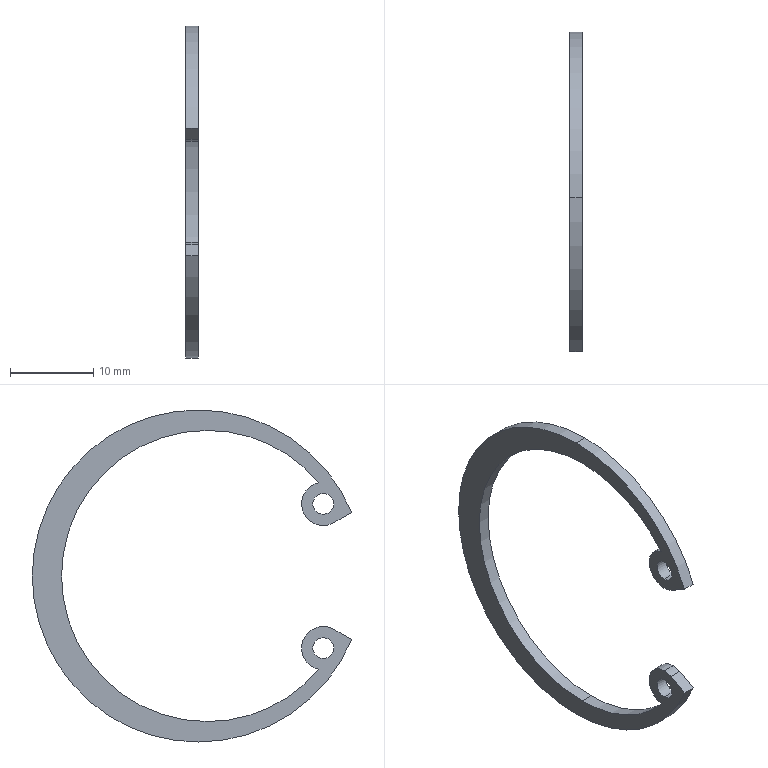Part | STEP file | RTWN37_RTWN37 | 1 solid | 17 faces | box 1.5 x 38.283 x 39.8 mm | volume 431.748 mm3 | cylinder 13 | plane 4 | commonest cylinder face diameters 2.5 x4 5.2 x3 34.9 x3 39.8 x3
STEP:
#1=CARTESIAN_POINT('',(0.,0.,0.));
#2=DIRECTION('',(0.,0.,1.));
#3=DIRECTION('',(1.,0.,0.));
#4=AXIS2_PLACEMENT_3D('',#1,#2,#3);
#5=CARTESIAN_POINT('',(0.75,-14.982,9.9));
#6=VERTEX_POINT('',#5);
#7=CARTESIAN_POINT('',(-0.75,-14.982,9.9));
#8=VERTEX_POINT('',#7);
#9=CARTESIAN_POINT('',(0.75,-14.982,9.9));
#10=DIRECTION('',(-1.,0.,0.));
#11=VECTOR('',#10,1.);
#12=LINE('',#9,#11);
#13=CARTESIAN_POINT('',(0.75,-14.982,8.65));
#14=DIRECTION('',(-1.,0.,0.));
#15=DIRECTION('',(0.,0.,1.));
#16=AXIS2_PLACEMENT_3D('',#13,#14,#15);
#17=CYLINDRICAL_SURFACE('',#16,1.25);
#18=CARTESIAN_POINT('',(6.283,0.));
#19=DIRECTION('',(0.,1.));
#20=VECTOR('',#19,1.);
#21=LINE('',#18,#20);
#22=(GEOMETRIC_REPRESENTATION_CONTEXT(2)PARAMETRIC_REPRESENTATION_CONTEXT()REPRESENTATION_CONTEXT('',''));
#23=DEFINITIONAL_REPRESENTATION('',(#21),#22);
#24=PCURVE('',#17,#23);
#25=CARTESIAN_POINT('',(0.75,-14.982,8.65));
#26=DIRECTION('',(-1.,0.,0.));
#27=DIRECTION('',(0.,0.,1.));
#28=AXIS2_PLACEMENT_3D('',#25,#26,#27);
#29=CYLINDRICAL_SURFACE('',#28,1.25);
#30=CARTESIAN_POINT('',(0.,0.));
#31=DIRECTION('',(0.,1.));
#32=VECTOR('',#31,1.);
#33=LINE('',#30,#32);
#34=(GEOMETRIC_REPRESENTATION_CONTEXT(2)PARAMETRIC_REPRESENTATION_CONTEXT()REPRESENTATION_CONTEXT('',''));
#35=DEFINITIONAL_REPRESENTATION('',(#33),#34);
#36=PCURVE('',#29,#35);
#37=SURFACE_CURVE('',#12,(#24,#36),.PCURVE_S1.);
#38=EDGE_CURVE('',#6,#8,#37,.T.);
#39=ORIENTED_EDGE('',*,*,#38,.T.);
#40=CARTESIAN_POINT('',(-0.75,-14.982,7.4));
#41=VERTEX_POINT('',#40);
#42=CARTESIAN_POINT('',(-0.75,-14.982,8.65));
#43=DIRECTION('',(1.,0.,0.));
#44=DIRECTION('',(0.,0.,-1.));
#45=AXIS2_PLACEMENT_3D('',#42,#43,#44);
#46=CIRCLE('',#45,1.25);
#47=CARTESIAN_POINT('',(9.425,1.5));
#48=DIRECTION('',(-1.,0.));
#49=VECTOR('',#48,1.);
#50=LINE('',#47,#49);
#51=(GEOMETRIC_REPRESENTATION_CONTEXT(2)PARAMETRIC_REPRESENTATION_CONTEXT()REPRESENTATION_CONTEXT('',''));
#52=DEFINITIONAL_REPRESENTATION('',(#50),#51);
#53=PCURVE('',#17,#52);
#54=CARTESIAN_POINT('',(-0.75,0.,0.));
#55=DIRECTION('',(1.,0.,0.));
#56=DIRECTION('',(0.,0.,-1.));
#57=AXIS2_PLACEMENT_3D('',#54,#55,#56);
#58=PLANE('',#57);
#59=CARTESIAN_POINT('',(-8.65,-14.982));
#60=DIRECTION('',(1.,0.));
#61=AXIS2_PLACEMENT_2D('',#59,#60);
#62=CIRCLE('',#61,1.25);
#63=(GEOMETRIC_REPRESENTATION_CONTEXT(2)PARAMETRIC_REPRESENTATION_CONTEXT()REPRESENTATION_CONTEXT('',''));
#64=DEFINITIONAL_REPRESENTATION('',(#62),#63);
#65=PCURVE('',#58,#64);
#66=SURFACE_CURVE('',#46,(#53,#65),.PCURVE_S1.);
#67=EDGE_CURVE('',#8,#41,#66,.T.);
#68=ORIENTED_EDGE('',*,*,#67,.T.);
#69=CARTESIAN_POINT('',(0.75,-14.982,7.4));
#70=VERTEX_POINT('',#69);
#71=CARTESIAN_POINT('',(0.75,-14.982,7.4));
#72=DIRECTION('',(-1.,0.,0.));
#73=VECTOR('',#72,1.);
#74=LINE('',#71,#73);
#75=CARTESIAN_POINT('',(3.142,0.));
#76=DIRECTION('',(0.,1.));
#77=VECTOR('',#76,1.);
#78=LINE('',#75,#77);
#79=(GEOMETRIC_REPRESENTATION_CONTEXT(2)PARAMETRIC_REPRESENTATION_CONTEXT()REPRESENTATION_CONTEXT('',''));
#80=DEFINITIONAL_REPRESENTATION('',(#78),#79);
#81=PCURVE('',#17,#80);
#82=CARTESIAN_POINT('',(3.142,0.));
#83=DIRECTION('',(0.,1.));
#84=VECTOR('',#83,1.);
#85=LINE('',#82,#84);
#86=(GEOMETRIC_REPRESENTATION_CONTEXT(2)PARAMETRIC_REPRESENTATION_CONTEXT()REPRESENTATION_CONTEXT('',''));
#87=DEFINITIONAL_REPRESENTATION('',(#85),#86);
#88=PCURVE('',#29,#87);
#89=SURFACE_CURVE('',#74,(#81,#88),.PCURVE_S1.);
#90=EDGE_CURVE('',#70,#41,#89,.T.);
#91=ORIENTED_EDGE('',*,*,#90,.F.);
#92=CARTESIAN_POINT('',(0.75,-14.982,8.65));
#93=DIRECTION('',(1.,0.,0.));
#94=DIRECTION('',(0.,0.,-1.));
#95=AXIS2_PLACEMENT_3D('',#92,#93,#94);
#96=CIRCLE('',#95,1.25);
#97=CARTESIAN_POINT('',(9.425,0.));
#98=DIRECTION('',(-1.,0.));
#99=VECTOR('',#98,1.);
#100=LINE('',#97,#99);
#101=(GEOMETRIC_REPRESENTATION_CONTEXT(2)PARAMETRIC_REPRESENTATION_CONTEXT()REPRESENTATION_CONTEXT('',''));
#102=DEFINITIONAL_REPRESENTATION('',(#100),#101);
#103=PCURVE('',#17,#102);
#104=CARTESIAN_POINT('',(0.75,0.,0.));
#105=DIRECTION('',(1.,0.,0.));
#106=DIRECTION('',(0.,0.,-1.));
#107=AXIS2_PLACEMENT_3D('',#104,#105,#106);
#108=PLANE('',#107);
#109=CARTESIAN_POINT('',(-8.65,-14.982));
#110=DIRECTION('',(1.,0.));
#111=AXIS2_PLACEMENT_2D('',#109,#110);
#112=CIRCLE('',#111,1.25);
#113=(GEOMETRIC_REPRESENTATION_CONTEXT(2)PARAMETRIC_REPRESENTATION_CONTEXT()REPRESENTATION_CONTEXT('',''));
#114=DEFINITIONAL_REPRESENTATION('',(#112),#113);
#115=PCURVE('',#108,#114);
#116=SURFACE_CURVE('',#96,(#103,#115),.PCURVE_S1.);
#117=EDGE_CURVE('',#6,#70,#116,.T.);
#118=ORIENTED_EDGE('',*,*,#117,.F.);
#119=EDGE_LOOP('',(#39,#68,#91,#118));
#120=FACE_BOUND('',#119,.F.);
#121=ADVANCED_FACE('',(#120),#17,.F.);
#122=CARTESIAN_POINT('',(0.75,-14.982,-7.4));
#123=VERTEX_POINT('',#122);
#124=CARTESIAN_POINT('',(-0.75,-14.982,-7.4));
#125=VERTEX_POINT('',#124);
#126=CARTESIAN_POINT('',(0.75,-14.982,-7.4));
#127=DIRECTION('',(-1.,0.,0.));
#128=VECTOR('',#127,1.);
#129=LINE('',#126,#128);
#130=CARTESIAN_POINT('',(0.75,-14.982,-8.65));
#131=DIRECTION('',(-1.,0.,0.));
#132=DIRECTION('',(0.,0.,1.));
#133=AXIS2_PLACEMENT_3D('',#130,#131,#132);
#134=CYLINDRICAL_SURFACE('',#133,1.25);
#135=CARTESIAN_POINT('',(6.283,0.));
#136=DIRECTION('',(0.,1.));
#137=VECTOR('',#136,1.);
#138=LINE('',#135,#137);
#139=(GEOMETRIC_REPRESENTATION_CONTEXT(2)PARAMETRIC_REPRESENTATION_CONTEXT()REPRESENTATION_CONTEXT('',''));
#140=DEFINITIONAL_REPRESENTATION('',(#138),#139);
#141=PCURVE('',#134,#140);
#142=CARTESIAN_POINT('',(0.75,-14.982,-8.65));
#143=DIRECTION('',(-1.,0.,0.));
#144=DIRECTION('',(0.,0.,1.));
#145=AXIS2_PLACEMENT_3D('',#142,#143,#144);
#146=CYLINDRICAL_SURFACE('',#145,1.25);
#147=CARTESIAN_POINT('',(0.,0.));
#148=DIRECTION('',(0.,1.));
#149=VECTOR('',#148,1.);
#150=LINE('',#147,#149);
#151=(GEOMETRIC_REPRESENTATION_CONTEXT(2)PARAMETRIC_REPRESENTATION_CONTEXT()REPRESENTATION_CONTEXT('',''));
#152=DEFINITIONAL_REPRESENTATION('',(#150),#151);
#153=PCURVE('',#146,#152);
#154=SURFACE_CURVE('',#129,(#141,#153),.PCURVE_S1.);
#155=EDGE_CURVE('',#123,#125,#154,.T.);
#156=ORIENTED_EDGE('',*,*,#155,.T.);
#157=CARTESIAN_POINT('',(-0.75,-14.982,-9.9));
#158=VERTEX_POINT('',#157);
#159=CARTESIAN_POINT('',(-0.75,-14.982,-8.65));
#160=DIRECTION('',(1.,0.,0.));
#161=DIRECTION('',(0.,0.,-1.));
#162=AXIS2_PLACEMENT_3D('',#159,#160,#161);
#163=CIRCLE('',#162,1.25);
#164=CARTESIAN_POINT('',(9.425,1.5));
#165=DIRECTION('',(-1.,0.));
#166=VECTOR('',#165,1.);
#167=LINE('',#164,#166);
#168=(GEOMETRIC_REPRESENTATION_CONTEXT(2)PARAMETRIC_REPRESENTATION_CONTEXT()REPRESENTATION_CONTEXT('',''));
#169=DEFINITIONAL_REPRESENTATION('',(#167),#168);
#170=PCURVE('',#134,#169);
#171=CARTESIAN_POINT('',(8.65,-14.982));
#172=DIRECTION('',(1.,0.));
#173=AXIS2_PLACEMENT_2D('',#171,#172);
#174=CIRCLE('',#173,1.25);
#175=(GEOMETRIC_REPRESENTATION_CONTEXT(2)PARAMETRIC_REPRESENTATION_CONTEXT()REPRESENTATION_CONTEXT('',''));
#176=DEFINITIONAL_REPRESENTATION('',(#174),#175);
#177=PCURVE('',#58,#176);
#178=SURFACE_CURVE('',#163,(#170,#177),.PCURVE_S1.);
#179=EDGE_CURVE('',#125,#158,#178,.T.);
#180=ORIENTED_EDGE('',*,*,#179,.T.);
#181=CARTESIAN_POINT('',(0.75,-14.982,-9.9));
#182=VERTEX_POINT('',#181);
#183=CARTESIAN_POINT('',(0.75,-14.982,-9.9));
#184=DIRECTION('',(-1.,0.,0.));
#185=VECTOR('',#184,1.);
#186=LINE('',#183,#185);
#187=CARTESIAN_POINT('',(3.142,0.));
#188=DIRECTION('',(0.,1.));
#189=VECTOR('',#188,1.);
#190=LINE('',#187,#189);
#191=(GEOMETRIC_REPRESENTATION_CONTEXT(2)PARAMETRIC_REPRESENTATION_CONTEXT()REPRESENTATION_CONTEXT('',''));
#192=DEFINITIONAL_REPRESENTATION('',(#190),#191);
#193=PCURVE('',#134,#192);
#194=CARTESIAN_POINT('',(3.142,0.));
#195=DIRECTION('',(0.,1.));
#196=VECTOR('',#195,1.);
#197=LINE('',#194,#196);
#198=(GEOMETRIC_REPRESENTATION_CONTEXT(2)PARAMETRIC_REPRESENTATION_CONTEXT()REPRESENTATION_CONTEXT('',''));
#199=DEFINITIONAL_REPRESENTATION('',(#197),#198);
#200=PCURVE('',#146,#199);
#201=SURFACE_CURVE('',#186,(#193,#200),.PCURVE_S1.);
#202=EDGE_CURVE('',#182,#158,#201,.T.);
#203=ORIENTED_EDGE('',*,*,#202,.F.);
#204=CARTESIAN_POINT('',(0.75,-14.982,-8.65));
#205=DIRECTION('',(1.,0.,0.));
#206=DIRECTION('',(0.,0.,-1.));
#207=AXIS2_PLACEMENT_3D('',#204,#205,#206);
#208=CIRCLE('',#207,1.25);
#209=CARTESIAN_POINT('',(9.425,0.));
#210=DIRECTION('',(-1.,0.));
#211=VECTOR('',#210,1.);
#212=LINE('',#209,#211);
#213=(GEOMETRIC_REPRESENTATION_CONTEXT(2)PARAMETRIC_REPRESENTATION_CONTEXT()REPRESENTATION_CONTEXT('',''));
#214=DEFINITIONAL_REPRESENTATION('',(#212),#213);
#215=PCURVE('',#134,#214);
#216=CARTESIAN_POINT('',(8.65,-14.982));
#217=DIRECTION('',(1.,0.));
#218=AXIS2_PLACEMENT_2D('',#216,#217);
#219=CIRCLE('',#218,1.25);
#220=(GEOMETRIC_REPRESENTATION_CONTEXT(2)PARAMETRIC_REPRESENTATION_CONTEXT()REPRESENTATION_CONTEXT('',''));
#221=DEFINITIONAL_REPRESENTATION('',(#219),#220);
#222=PCURVE('',#108,#221);
#223=SURFACE_CURVE('',#208,(#215,#222),.PCURVE_S1.);
#224=EDGE_CURVE('',#123,#182,#223,.T.);
#225=ORIENTED_EDGE('',*,*,#224,.F.);
#226=EDGE_LOOP('',(#156,#180,#203,#225));
#227=FACE_BOUND('',#226,.F.);
#228=ADVANCED_FACE('',(#227),#134,.F.);
#229=CARTESIAN_POINT('',(0.75,-14.982,-6.05));
#230=VERTEX_POINT('',#229);
#231=CARTESIAN_POINT('',(0.75,-16.109,-6.307));
#232=VERTEX_POINT('',#231);
#233=CARTESIAN_POINT('',(0.75,-14.982,-8.65));
#234=DIRECTION('',(1.,0.,0.));
#235=DIRECTION('',(0.,0.,-1.));
#236=AXIS2_PLACEMENT_3D('',#233,#234,#235);
#237=CIRCLE('',#236,2.6);
#238=CARTESIAN_POINT('',(0.75,-14.982,-8.65));
#239=DIRECTION('',(-1.,0.,0.));
#240=DIRECTION('',(0.,0.,1.));
#241=AXIS2_PLACEMENT_3D('',#238,#239,#240);
#242=CYLINDRICAL_SURFACE('',#241,2.6);
#243=CARTESIAN_POINT('',(9.425,0.));
#244=DIRECTION('',(-1.,0.));
#245=VECTOR('',#244,1.);
#246=LINE('',#243,#245);
#247=(GEOMETRIC_REPRESENTATION_CONTEXT(2)PARAMETRIC_REPRESENTATION_CONTEXT()REPRESENTATION_CONTEXT('',''));
#248=DEFINITIONAL_REPRESENTATION('',(#246),#247);
#249=PCURVE('',#242,#248);
#250=CARTESIAN_POINT('',(8.65,-14.982));
#251=DIRECTION('',(1.,0.));
#252=AXIS2_PLACEMENT_2D('',#250,#251);
#253=CIRCLE('',#252,2.6);
#254=(GEOMETRIC_REPRESENTATION_CONTEXT(2)PARAMETRIC_REPRESENTATION_CONTEXT()REPRESENTATION_CONTEXT('',''));
#255=DEFINITIONAL_REPRESENTATION('',(#253),#254);
#256=PCURVE('',#108,#255);
#257=SURFACE_CURVE('',#237,(#249,#256),.PCURVE_S1.);
#258=EDGE_CURVE('',#230,#232,#257,.T.);
#259=ORIENTED_EDGE('',*,*,#258,.F.);
#260=CARTESIAN_POINT('',(-0.75,-14.982,-6.05));
#261=VERTEX_POINT('',#260);
#262=CARTESIAN_POINT('',(0.75,-14.982,-6.05));
#263=DIRECTION('',(-1.,0.,0.));
#264=VECTOR('',#263,1.);
#265=LINE('',#262,#264);
#266=CARTESIAN_POINT('',(6.283,0.));
#267=DIRECTION('',(0.,1.));
#268=VECTOR('',#267,1.);
#269=LINE('',#266,#268);
#270=(GEOMETRIC_REPRESENTATION_CONTEXT(2)PARAMETRIC_REPRESENTATION_CONTEXT()REPRESENTATION_CONTEXT('',''));
#271=DEFINITIONAL_REPRESENTATION('',(#269),#270);
#272=PCURVE('',#242,#271);
#273=CARTESIAN_POINT('',(0.75,-14.982,-8.65));
#274=DIRECTION('',(-1.,0.,0.));
#275=DIRECTION('',(0.,0.,1.));
#276=AXIS2_PLACEMENT_3D('',#273,#274,#275);
#277=CYLINDRICAL_SURFACE('',#276,2.6);
#278=CARTESIAN_POINT('',(0.,0.));
#279=DIRECTION('',(0.,1.));
#280=VECTOR('',#279,1.);
#281=LINE('',#278,#280);
#282=(GEOMETRIC_REPRESENTATION_CONTEXT(2)PARAMETRIC_REPRESENTATION_CONTEXT()REPRESENTATION_CONTEXT('',''));
#283=DEFINITIONAL_REPRESENTATION('',(#281),#282);
#284=PCURVE('',#277,#283);
#285=SURFACE_CURVE('',#265,(#272,#284),.PCURVE_S1.);
#286=EDGE_CURVE('',#230,#261,#285,.T.);
#287=ORIENTED_EDGE('',*,*,#286,.T.);
#288=CARTESIAN_POINT('',(-0.75,-16.109,-6.307));
#289=VERTEX_POINT('',#288);
#290=CARTESIAN_POINT('',(-0.75,-14.982,-8.65));
#291=DIRECTION('',(1.,0.,0.));
#292=DIRECTION('',(0.,0.,-1.));
#293=AXIS2_PLACEMENT_3D('',#290,#291,#292);
#294=CIRCLE('',#293,2.6);
#295=CARTESIAN_POINT('',(9.425,1.5));
#296=DIRECTION('',(-1.,0.));
#297=VECTOR('',#296,1.);
#298=LINE('',#295,#297);
#299=(GEOMETRIC_REPRESENTATION_CONTEXT(2)PARAMETRIC_REPRESENTATION_CONTEXT()REPRESENTATION_CONTEXT('',''));
#300=DEFINITIONAL_REPRESENTATION('',(#298),#299);
#301=PCURVE('',#242,#300);
#302=CARTESIAN_POINT('',(8.65,-14.982));
#303=DIRECTION('',(1.,0.));
#304=AXIS2_PLACEMENT_2D('',#302,#303);
#305=CIRCLE('',#304,2.6);
#306=(GEOMETRIC_REPRESENTATION_CONTEXT(2)PARAMETRIC_REPRESENTATION_CONTEXT()REPRESENTATION_CONTEXT('',''));
#307=DEFINITIONAL_REPRESENTATION('',(#305),#306);
#308=PCURVE('',#58,#307);
#309=SURFACE_CURVE('',#294,(#301,#308),.PCURVE_S1.);
#310=EDGE_CURVE('',#261,#289,#309,.T.);
#311=ORIENTED_EDGE('',*,*,#310,.T.);
#312=CARTESIAN_POINT('',(0.75,-16.109,-6.307));
#313=DIRECTION('',(-1.,0.,0.));
#314=VECTOR('',#313,1.);
#315=LINE('',#312,#314);
#316=CARTESIAN_POINT('',(5.835,0.));
#317=DIRECTION('',(0.,1.));
#318=VECTOR('',#317,1.);
#319=LINE('',#316,#318);
#320=(GEOMETRIC_REPRESENTATION_CONTEXT(2)PARAMETRIC_REPRESENTATION_CONTEXT()REPRESENTATION_CONTEXT('',''));
#321=DEFINITIONAL_REPRESENTATION('',(#319),#320);
#322=PCURVE('',#242,#321);
#323=CARTESIAN_POINT('',(0.75,-16.109,-6.307));
#324=DIRECTION('',(0.,0.5,-0.866));
#325=DIRECTION('',(0.,0.866,0.5));
#326=AXIS2_PLACEMENT_3D('',#323,#324,#325);
#327=PLANE('',#326);
#328=CARTESIAN_POINT('',(0.,0.));
#329=DIRECTION('',(0.,-1.));
#330=VECTOR('',#329,1.);
#331=LINE('',#328,#330);
#332=(GEOMETRIC_REPRESENTATION_CONTEXT(2)PARAMETRIC_REPRESENTATION_CONTEXT()REPRESENTATION_CONTEXT('',''));
#333=DEFINITIONAL_REPRESENTATION('',(#331),#332);
#334=PCURVE('',#327,#333);
#335=SURFACE_CURVE('',#315,(#322,#334),.PCURVE_S1.);
#336=EDGE_CURVE('',#232,#289,#335,.T.);
#337=ORIENTED_EDGE('',*,*,#336,.F.);
#338=EDGE_LOOP('',(#259,#287,#311,#337));
#339=FACE_BOUND('',#338,.T.);
#340=ADVANCED_FACE('',(#339),#242,.T.);
#341=CARTESIAN_POINT('',(0.75,-14.438,-11.192));
#342=VERTEX_POINT('',#341);
#343=CARTESIAN_POINT('',(-0.75,-14.438,-11.192));
#344=VERTEX_POINT('',#343);
#345=CARTESIAN_POINT('',(0.75,-14.438,-11.192));
#346=DIRECTION('',(-1.,0.,0.));
#347=VECTOR('',#346,1.);
#348=LINE('',#345,#347);
#349=CARTESIAN_POINT('',(0.75,-1.05,0.));
#350=DIRECTION('',(-1.,0.,0.));
#351=DIRECTION('',(0.,0.,1.));
#352=AXIS2_PLACEMENT_3D('',#349,#350,#351);
#353=CYLINDRICAL_SURFACE('',#352,17.45);
#354=CARTESIAN_POINT('',(4.016,0.));
#355=DIRECTION('',(0.,1.));
#356=VECTOR('',#355,1.);
#357=LINE('',#354,#356);
#358=(GEOMETRIC_REPRESENTATION_CONTEXT(2)PARAMETRIC_REPRESENTATION_CONTEXT()REPRESENTATION_CONTEXT('',''));
#359=DEFINITIONAL_REPRESENTATION('',(#357),#358);
#360=PCURVE('',#353,#359);
#361=CARTESIAN_POINT('',(2.931,0.));
#362=DIRECTION('',(0.,1.));
#363=VECTOR('',#362,1.);
#364=LINE('',#361,#363);
#365=(GEOMETRIC_REPRESENTATION_CONTEXT(2)PARAMETRIC_REPRESENTATION_CONTEXT()REPRESENTATION_CONTEXT('',''));
#366=DEFINITIONAL_REPRESENTATION('',(#364),#365);
#367=PCURVE('',#277,#366);
#368=SURFACE_CURVE('',#348,(#360,#367),.PCURVE_S1.);
#369=EDGE_CURVE('',#342,#344,#368,.T.);
#370=ORIENTED_EDGE('',*,*,#369,.T.);
#371=CARTESIAN_POINT('',(-0.75,-1.05,-17.45));
#372=VERTEX_POINT('',#371);
#373=CARTESIAN_POINT('',(-0.75,-1.05,0.));
#374=DIRECTION('',(-1.,0.,0.));
#375=DIRECTION('',(0.,0.,1.));
#376=AXIS2_PLACEMENT_3D('',#373,#374,#375);
#377=CIRCLE('',#376,17.45);
#378=CARTESIAN_POINT('',(0.,1.5));
#379=DIRECTION('',(1.,0.));
#380=VECTOR('',#379,1.);
#381=LINE('',#378,#380);
#382=(GEOMETRIC_REPRESENTATION_CONTEXT(2)PARAMETRIC_REPRESENTATION_CONTEXT()REPRESENTATION_CONTEXT('',''));
#383=DEFINITIONAL_REPRESENTATION('',(#381),#382);
#384=PCURVE('',#353,#383);
#385=CARTESIAN_POINT('',(-17.45,-1.05));
#386=CARTESIAN_POINT('',(-17.45,29.174));
#387=CARTESIAN_POINT('',(8.725,14.062));
#388=CARTESIAN_POINT('',(34.9,-1.05));
#389=CARTESIAN_POINT('',(8.725,-16.162));
#390=CARTESIAN_POINT('',(-17.45,-31.274));
#391=CARTESIAN_POINT('',(-17.45,-1.05));
#392=(BOUNDED_CURVE()B_SPLINE_CURVE(2,(#385,#386,#387,#388,#389,#390,#391),.UNSPECIFIED.,.T.,.F.)B_SPLINE_CURVE_WITH_KNOTS((1,2,2,2,2,1),(-2.094,0.,2.094,4.189,6.283,8.378),.UNSPECIFIED.)CURVE()GEOMETRIC_REPRESENTATION_ITEM()RATIONAL_B_SPLINE_CURVE((1.,0.5,1.,0.5,1.,0.5,1.))REPRESENTATION_ITEM(''));
#393=(GEOMETRIC_REPRESENTATION_CONTEXT(2)PARAMETRIC_REPRESENTATION_CONTEXT()REPRESENTATION_CONTEXT('',''));
#394=DEFINITIONAL_REPRESENTATION('',(#392),#393);
#395=PCURVE('',#58,#394);
#396=SURFACE_CURVE('',#377,(#384,#395),.PCURVE_S1.);
#397=EDGE_CURVE('',#372,#344,#396,.T.);
#398=ORIENTED_EDGE('',*,*,#397,.F.);
#399=CARTESIAN_POINT('',(0.75,-1.05,-17.45));
#400=VERTEX_POINT('',#399);
#401=CARTESIAN_POINT('',(0.75,-1.05,-17.45));
#402=DIRECTION('',(-1.,0.,0.));
#403=VECTOR('',#402,1.);
#404=LINE('',#401,#403);
#405=CARTESIAN_POINT('',(3.142,0.));
#406=DIRECTION('',(0.,1.));
#407=VECTOR('',#406,1.);
#408=LINE('',#405,#407);
#409=(GEOMETRIC_REPRESENTATION_CONTEXT(2)PARAMETRIC_REPRESENTATION_CONTEXT()REPRESENTATION_CONTEXT('',''));
#410=DEFINITIONAL_REPRESENTATION('',(#408),#409);
#411=PCURVE('',#353,#410);
#412=CARTESIAN_POINT('',(0.75,-1.05,0.));
#413=DIRECTION('',(-1.,0.,0.));
#414=DIRECTION('',(0.,0.,1.));
#415=AXIS2_PLACEMENT_3D('',#412,#413,#414);
#416=CYLINDRICAL_SURFACE('',#415,17.45);
#417=CARTESIAN_POINT('',(3.142,0.));
#418=DIRECTION('',(0.,1.));
#419=VECTOR('',#418,1.);
#420=LINE('',#417,#419);
#421=(GEOMETRIC_REPRESENTATION_CONTEXT(2)PARAMETRIC_REPRESENTATION_CONTEXT()REPRESENTATION_CONTEXT('',''));
#422=DEFINITIONAL_REPRESENTATION('',(#420),#421);
#423=PCURVE('',#416,#422);
#424=SURFACE_CURVE('',#404,(#411,#423),.PCURVE_S1.);
#425=EDGE_CURVE('',#400,#372,#424,.T.);
#426=ORIENTED_EDGE('',*,*,#425,.F.);
#427=CARTESIAN_POINT('',(0.75,-1.05,0.));
#428=DIRECTION('',(-1.,0.,0.));
#429=DIRECTION('',(0.,0.,1.));
#430=AXIS2_PLACEMENT_3D('',#427,#428,#429);
#431=CIRCLE('',#430,17.45);
#432=CARTESIAN_POINT('',(0.,0.));
#433=DIRECTION('',(1.,0.));
#434=VECTOR('',#433,1.);
#435=LINE('',#432,#434);
#436=(GEOMETRIC_REPRESENTATION_CONTEXT(2)PARAMETRIC_REPRESENTATION_CONTEXT()REPRESENTATION_CONTEXT('',''));
#437=DEFINITIONAL_REPRESENTATION('',(#435),#436);
#438=PCURVE('',#353,#437);
#439=CARTESIAN_POINT('',(-17.45,-1.05));
#440=CARTESIAN_POINT('',(-17.45,29.174));
#441=CARTESIAN_POINT('',(8.725,14.062));
#442=CARTESIAN_POINT('',(34.9,-1.05));
#443=CARTESIAN_POINT('',(8.725,-16.162));
#444=CARTESIAN_POINT('',(-17.45,-31.274));
#445=CARTESIAN_POINT('',(-17.45,-1.05));
#446=(BOUNDED_CURVE()B_SPLINE_CURVE(2,(#439,#440,#441,#442,#443,#444,#445),.UNSPECIFIED.,.T.,.F.)B_SPLINE_CURVE_WITH_KNOTS((1,2,2,2,2,1),(-2.094,0.,2.094,4.189,6.283,8.378),.UNSPECIFIED.)CURVE()GEOMETRIC_REPRESENTATION_ITEM()RATIONAL_B_SPLINE_CURVE((1.,0.5,1.,0.5,1.,0.5,1.))REPRESENTATION_ITEM(''));
#447=(GEOMETRIC_REPRESENTATION_CONTEXT(2)PARAMETRIC_REPRESENTATION_CONTEXT()REPRESENTATION_CONTEXT('',''));
#448=DEFINITIONAL_REPRESENTATION('',(#446),#447);
#449=PCURVE('',#108,#448);
#450=SURFACE_CURVE('',#431,(#438,#449),.PCURVE_S1.);
#451=EDGE_CURVE('',#400,#342,#450,.T.);
#452=ORIENTED_EDGE('',*,*,#451,.T.);
#453=EDGE_LOOP('',(#370,#398,#426,#452));
#454=FACE_BOUND('',#453,.F.);
#455=ADVANCED_FACE('',(#454),#353,.F.);
#456=CARTESIAN_POINT('',(-0.75,-1.05,17.45));
#457=VERTEX_POINT('',#456);
#458=CARTESIAN_POINT('',(-0.75,-1.05,0.));
#459=DIRECTION('',(-1.,0.,0.));
#460=DIRECTION('',(0.,0.,1.));
#461=AXIS2_PLACEMENT_3D('',#458,#459,#460);
#462=CIRCLE('',#461,17.45);
#463=CARTESIAN_POINT('',(0.,1.5));
#464=DIRECTION('',(1.,0.));
#465=VECTOR('',#464,1.);
#466=LINE('',#463,#465);
#467=(GEOMETRIC_REPRESENTATION_CONTEXT(2)PARAMETRIC_REPRESENTATION_CONTEXT()REPRESENTATION_CONTEXT('',''));
#468=DEFINITIONAL_REPRESENTATION('',(#466),#467);
#469=PCURVE('',#416,#468);
#470=CARTESIAN_POINT('',(-17.45,-1.05));
#471=CARTESIAN_POINT('',(-17.45,29.174));
#472=CARTESIAN_POINT('',(8.725,14.062));
#473=CARTESIAN_POINT('',(34.9,-1.05));
#474=CARTESIAN_POINT('',(8.725,-16.162));
#475=CARTESIAN_POINT('',(-17.45,-31.274));
#476=CARTESIAN_POINT('',(-17.45,-1.05));
#477=(BOUNDED_CURVE()B_SPLINE_CURVE(2,(#470,#471,#472,#473,#474,#475,#476),.UNSPECIFIED.,.T.,.F.)B_SPLINE_CURVE_WITH_KNOTS((1,2,2,2,2,1),(-2.094,0.,2.094,4.189,6.283,8.378),.UNSPECIFIED.)CURVE()GEOMETRIC_REPRESENTATION_ITEM()RATIONAL_B_SPLINE_CURVE((1.,0.5,1.,0.5,1.,0.5,1.))REPRESENTATION_ITEM(''));
#478=(GEOMETRIC_REPRESENTATION_CONTEXT(2)PARAMETRIC_REPRESENTATION_CONTEXT()REPRESENTATION_CONTEXT('',''));
#479=DEFINITIONAL_REPRESENTATION('',(#477),#478);
#480=PCURVE('',#58,#479);
#481=SURFACE_CURVE('',#462,(#469,#480),.PCURVE_S1.);
#482=EDGE_CURVE('',#457,#372,#481,.T.);
#483=ORIENTED_EDGE('',*,*,#482,.F.);
#484=CARTESIAN_POINT('',(0.75,-1.05,17.45));
#485=VERTEX_POINT('',#484);
#486=CARTESIAN_POINT('',(0.75,-1.05,17.45));
#487=DIRECTION('',(-1.,0.,0.));
#488=VECTOR('',#487,1.);
#489=LINE('',#486,#488);
#490=CARTESIAN_POINT('',(0.,0.));
#491=DIRECTION('',(0.,1.));
#492=VECTOR('',#491,1.);
#493=LINE('',#490,#492);
#494=(GEOMETRIC_REPRESENTATION_CONTEXT(2)PARAMETRIC_REPRESENTATION_CONTEXT()REPRESENTATION_CONTEXT('',''));
#495=DEFINITIONAL_REPRESENTATION('',(#493),#494);
#496=PCURVE('',#416,#495);
#497=CARTESIAN_POINT('',(0.75,-1.05,0.));
#498=DIRECTION('',(-1.,0.,0.));
#499=DIRECTION('',(0.,0.,1.));
#500=AXIS2_PLACEMENT_3D('',#497,#498,#499);
#501=CYLINDRICAL_SURFACE('',#500,17.45);
#502=CARTESIAN_POINT('',(6.283,0.));
#503=DIRECTION('',(0.,1.));
#504=VECTOR('',#503,1.);
#505=LINE('',#502,#504);
#506=(GEOMETRIC_REPRESENTATION_CONTEXT(2)PARAMETRIC_REPRESENTATION_CONTEXT()REPRESENTATION_CONTEXT('',''));
#507=DEFINITIONAL_REPRESENTATION('',(#505),#506);
#508=PCURVE('',#501,#507);
#509=SURFACE_CURVE('',#489,(#496,#508),.PCURVE_S1.);
#510=EDGE_CURVE('',#485,#457,#509,.T.);
#511=ORIENTED_EDGE('',*,*,#510,.F.);
#512=CARTESIAN_POINT('',(0.75,-1.05,0.));
#513=DIRECTION('',(-1.,0.,0.));
#514=DIRECTION('',(0.,0.,1.));
#515=AXIS2_PLACEMENT_3D('',#512,#513,#514);
#516=CIRCLE('',#515,17.45);
#517=CARTESIAN_POINT('',(0.,0.));
#518=DIRECTION('',(1.,0.));
#519=VECTOR('',#518,1.);
#520=LINE('',#517,#519);
#521=(GEOMETRIC_REPRESENTATION_CONTEXT(2)PARAMETRIC_REPRESENTATION_CONTEXT()REPRESENTATION_CONTEXT('',''));
#522=DEFINITIONAL_REPRESENTATION('',(#520),#521);
#523=PCURVE('',#416,#522);
#524=CARTESIAN_POINT('',(-17.45,-1.05));
#525=CARTESIAN_POINT('',(-17.45,29.174));
#526=CARTESIAN_POINT('',(8.725,14.062));
#527=CARTESIAN_POINT('',(34.9,-1.05));
#528=CARTESIAN_POINT('',(8.725,-16.162));
#529=CARTESIAN_POINT('',(-17.45,-31.274));
#530=CARTESIAN_POINT('',(-17.45,-1.05));
#531=(BOUNDED_CURVE()B_SPLINE_CURVE(2,(#524,#525,#526,#527,#528,#529,#530),.UNSPECIFIED.,.T.,.F.)B_SPLINE_CURVE_WITH_KNOTS((1,2,2,2,2,1),(-2.094,0.,2.094,4.189,6.283,8.378),.UNSPECIFIED.)CURVE()GEOMETRIC_REPRESENTATION_ITEM()RATIONAL_B_SPLINE_CURVE((1.,0.5,1.,0.5,1.,0.5,1.))REPRESENTATION_ITEM(''));
#532=(GEOMETRIC_REPRESENTATION_CONTEXT(2)PARAMETRIC_REPRESENTATION_CONTEXT()REPRESENTATION_CONTEXT('',''));
#533=DEFINITIONAL_REPRESENTATION('',(#531),#532);
#534=PCURVE('',#108,#533);
#535=SURFACE_CURVE('',#516,(#523,#534),.PCURVE_S1.);
#536=EDGE_CURVE('',#485,#400,#535,.T.);
#537=ORIENTED_EDGE('',*,*,#536,.T.);
#538=ORIENTED_EDGE('',*,*,#425,.T.);
#539=EDGE_LOOP('',(#483,#511,#537,#538));
#540=FACE_BOUND('',#539,.F.);
#541=ADVANCED_FACE('',(#540),#416,.F.);
#542=CARTESIAN_POINT('',(0.75,0.,-19.9));
#543=VERTEX_POINT('',#542);
#544=CARTESIAN_POINT('',(0.75,0.,19.9));
#545=VERTEX_POINT('',#544);
#546=CARTESIAN_POINT('',(0.75,0.,0.));
#547=DIRECTION('',(1.,0.,0.));
#548=DIRECTION('',(0.,0.,-1.));
#549=AXIS2_PLACEMENT_3D('',#546,#547,#548);
#550=CIRCLE('',#549,19.9);
#551=CARTESIAN_POINT('',(0.75,0.,0.));
#552=DIRECTION('',(-1.,0.,0.));
#553=DIRECTION('',(0.,0.,1.));
#554=AXIS2_PLACEMENT_3D('',#551,#552,#553);
#555=CYLINDRICAL_SURFACE('',#554,19.9);
#556=CARTESIAN_POINT('',(3.142,0.));
#557=DIRECTION('',(-1.,0.));
#558=VECTOR('',#557,1.);
#559=LINE('',#556,#558);
#560=(GEOMETRIC_REPRESENTATION_CONTEXT(2)PARAMETRIC_REPRESENTATION_CONTEXT()REPRESENTATION_CONTEXT('',''));
#561=DEFINITIONAL_REPRESENTATION('',(#559),#560);
#562=PCURVE('',#555,#561);
#563=CARTESIAN_POINT('',(0.,0.));
#564=DIRECTION('',(1.,0.));
#565=AXIS2_PLACEMENT_2D('',#563,#564);
#566=CIRCLE('',#565,19.9);
#567=(GEOMETRIC_REPRESENTATION_CONTEXT(2)PARAMETRIC_REPRESENTATION_CONTEXT()REPRESENTATION_CONTEXT('',''));
#568=DEFINITIONAL_REPRESENTATION('',(#566),#567);
#569=PCURVE('',#108,#568);
#570=SURFACE_CURVE('',#550,(#562,#569),.PCURVE_S1.);
#571=EDGE_CURVE('',#543,#545,#570,.T.);
#572=ORIENTED_EDGE('',*,*,#571,.F.);
#573=CARTESIAN_POINT('',(-0.75,0.,-19.9));
#574=VERTEX_POINT('',#573);
#575=CARTESIAN_POINT('',(0.75,0.,-19.9));
#576=DIRECTION('',(-1.,0.,0.));
#577=VECTOR('',#576,1.);
#578=LINE('',#575,#577);
#579=CARTESIAN_POINT('',(3.142,0.));
#580=DIRECTION('',(0.,1.));
#581=VECTOR('',#580,1.);
#582=LINE('',#579,#581);
#583=(GEOMETRIC_REPRESENTATION_CONTEXT(2)PARAMETRIC_REPRESENTATION_CONTEXT()REPRESENTATION_CONTEXT('',''));
#584=DEFINITIONAL_REPRESENTATION('',(#582),#583);
#585=PCURVE('',#555,#584);
#586=CARTESIAN_POINT('',(0.75,0.,0.));
#587=DIRECTION('',(-1.,0.,0.));
#588=DIRECTION('',(0.,0.,1.));
#589=AXIS2_PLACEMENT_3D('',#586,#587,#588);
#590=CYLINDRICAL_SURFACE('',#589,19.9);
#591=CARTESIAN_POINT('',(3.142,0.));
#592=DIRECTION('',(0.,1.));
#593=VECTOR('',#592,1.);
#594=LINE('',#591,#593);
#595=(GEOMETRIC_REPRESENTATION_CONTEXT(2)PARAMETRIC_REPRESENTATION_CONTEXT()REPRESENTATION_CONTEXT('',''));
#596=DEFINITIONAL_REPRESENTATION('',(#594),#595);
#597=PCURVE('',#590,#596);
#598=SURFACE_CURVE('',#578,(#585,#597),.PCURVE_S1.);
#599=EDGE_CURVE('',#543,#574,#598,.T.);
#600=ORIENTED_EDGE('',*,*,#599,.T.);
#601=CARTESIAN_POINT('',(-0.75,0.,19.9));
#602=VERTEX_POINT('',#601);
#603=CARTESIAN_POINT('',(-0.75,0.,0.));
#604=DIRECTION('',(1.,0.,0.));
#605=DIRECTION('',(0.,0.,-1.));
#606=AXIS2_PLACEMENT_3D('',#603,#604,#605);
#607=CIRCLE('',#606,19.9);
#608=CARTESIAN_POINT('',(3.142,1.5));
#609=DIRECTION('',(-1.,0.));
#610=VECTOR('',#609,1.);
#611=LINE('',#608,#610);
#612=(GEOMETRIC_REPRESENTATION_CONTEXT(2)PARAMETRIC_REPRESENTATION_CONTEXT()REPRESENTATION_CONTEXT('',''));
#613=DEFINITIONAL_REPRESENTATION('',(#611),#612);
#614=PCURVE('',#555,#613);
#615=CARTESIAN_POINT('',(0.,0.));
#616=DIRECTION('',(1.,0.));
#617=AXIS2_PLACEMENT_2D('',#615,#616);
#618=CIRCLE('',#617,19.9);
#619=(GEOMETRIC_REPRESENTATION_CONTEXT(2)PARAMETRIC_REPRESENTATION_CONTEXT()REPRESENTATION_CONTEXT('',''));
#620=DEFINITIONAL_REPRESENTATION('',(#618),#619);
#621=PCURVE('',#58,#620);
#622=SURFACE_CURVE('',#607,(#614,#621),.PCURVE_S1.);
#623=EDGE_CURVE('',#574,#602,#622,.T.);
#624=ORIENTED_EDGE('',*,*,#623,.T.);
#625=CARTESIAN_POINT('',(0.75,0.,19.9));
#626=DIRECTION('',(-1.,0.,0.));
#627=VECTOR('',#626,1.);
#628=LINE('',#625,#627);
#629=CARTESIAN_POINT('',(0.,0.));
#630=DIRECTION('',(0.,1.));
#631=VECTOR('',#630,1.);
#632=LINE('',#629,#631);
#633=(GEOMETRIC_REPRESENTATION_CONTEXT(2)PARAMETRIC_REPRESENTATION_CONTEXT()REPRESENTATION_CONTEXT('',''));
#634=DEFINITIONAL_REPRESENTATION('',(#632),#633);
#635=PCURVE('',#555,#634);
#636=CARTESIAN_POINT('',(0.75,0.,0.));
#637=DIRECTION('',(-1.,0.,0.));
#638=DIRECTION('',(0.,0.,1.));
#639=AXIS2_PLACEMENT_3D('',#636,#637,#638);
#640=CYLINDRICAL_SURFACE('',#639,19.9);
#641=CARTESIAN_POINT('',(6.283,0.));
#642=DIRECTION('',(0.,1.));
#643=VECTOR('',#642,1.);
#644=LINE('',#641,#643);
#645=(GEOMETRIC_REPRESENTATION_CONTEXT(2)PARAMETRIC_REPRESENTATION_CONTEXT()REPRESENTATION_CONTEXT('',''));
#646=DEFINITIONAL_REPRESENTATION('',(#644),#645);
#647=PCURVE('',#640,#646);
#648=SURFACE_CURVE('',#628,(#635,#647),.PCURVE_S1.);
#649=EDGE_CURVE('',#545,#602,#648,.T.);
#650=ORIENTED_EDGE('',*,*,#649,.F.);
#651=EDGE_LOOP('',(#572,#600,#624,#650));
#652=FACE_BOUND('',#651,.T.);
#653=ADVANCED_FACE('',(#652),#555,.T.);
#654=CARTESIAN_POINT('',(0.75,-18.383,7.62));
#655=VERTEX_POINT('',#654);
#656=CARTESIAN_POINT('',(0.75,0.,0.));
#657=DIRECTION('',(1.,0.,0.));
#658=DIRECTION('',(0.,0.,-1.));
#659=AXIS2_PLACEMENT_3D('',#656,#657,#658);
#660=CIRCLE('',#659,19.9);
#661=CARTESIAN_POINT('',(9.425,0.));
#662=DIRECTION('',(-1.,0.));
#663=VECTOR('',#662,1.);
#664=LINE('',#661,#663);
#665=(GEOMETRIC_REPRESENTATION_CONTEXT(2)PARAMETRIC_REPRESENTATION_CONTEXT()REPRESENTATION_CONTEXT('',''));
#666=DEFINITIONAL_REPRESENTATION('',(#664),#665);
#667=PCURVE('',#640,#666);
#668=CARTESIAN_POINT('',(0.,0.));
#669=DIRECTION('',(1.,0.));
#670=AXIS2_PLACEMENT_2D('',#668,#669);
#671=CIRCLE('',#670,19.9);
#672=(GEOMETRIC_REPRESENTATION_CONTEXT(2)PARAMETRIC_REPRESENTATION_CONTEXT()REPRESENTATION_CONTEXT('',''));
#673=DEFINITIONAL_REPRESENTATION('',(#671),#672);
#674=PCURVE('',#108,#673);
#675=SURFACE_CURVE('',#660,(#667,#674),.PCURVE_S1.);
#676=EDGE_CURVE('',#545,#655,#675,.T.);
#677=ORIENTED_EDGE('',*,*,#676,.F.);
#678=ORIENTED_EDGE('',*,*,#649,.T.);
#679=CARTESIAN_POINT('',(-0.75,-18.383,7.62));
#680=VERTEX_POINT('',#679);
#681=CARTESIAN_POINT('',(-0.75,0.,0.));
#682=DIRECTION('',(1.,0.,0.));
#683=DIRECTION('',(0.,0.,-1.));
#684=AXIS2_PLACEMENT_3D('',#681,#682,#683);
#685=CIRCLE('',#684,19.9);
#686=CARTESIAN_POINT('',(9.425,1.5));
#687=DIRECTION('',(-1.,0.));
#688=VECTOR('',#687,1.);
#689=LINE('',#686,#688);
#690=(GEOMETRIC_REPRESENTATION_CONTEXT(2)PARAMETRIC_REPRESENTATION_CONTEXT()REPRESENTATION_CONTEXT('',''));
#691=DEFINITIONAL_REPRESENTATION('',(#689),#690);
#692=PCURVE('',#640,#691);
#693=CARTESIAN_POINT('',(0.,0.));
#694=DIRECTION('',(1.,0.));
#695=AXIS2_PLACEMENT_2D('',#693,#694);
#696=CIRCLE('',#695,19.9);
#697=(GEOMETRIC_REPRESENTATION_CONTEXT(2)PARAMETRIC_REPRESENTATION_CONTEXT()REPRESENTATION_CONTEXT('',''));
#698=DEFINITIONAL_REPRESENTATION('',(#696),#697);
#699=PCURVE('',#58,#698);
#700=SURFACE_CURVE('',#685,(#692,#699),.PCURVE_S1.);
#701=EDGE_CURVE('',#602,#680,#700,.T.);
#702=ORIENTED_EDGE('',*,*,#701,.T.);
#703=CARTESIAN_POINT('',(0.75,-18.383,7.62));
#704=DIRECTION('',(-1.,0.,0.));
#705=VECTOR('',#704,1.);
#706=LINE('',#703,#705);
#707=CARTESIAN_POINT('',(5.105,0.));
#708=DIRECTION('',(0.,1.));
#709=VECTOR('',#708,1.);
#710=LINE('',#707,#709);
#711=(GEOMETRIC_REPRESENTATION_CONTEXT(2)PARAMETRIC_REPRESENTATION_CONTEXT()REPRESENTATION_CONTEXT('',''));
#712=DEFINITIONAL_REPRESENTATION('',(#710),#711);
#713=PCURVE('',#640,#712);
#714=CARTESIAN_POINT('',(0.75,-18.383,7.62));
#715=DIRECTION('',(0.,0.5,0.866));
#716=DIRECTION('',(0.,-0.866,0.5));
#717=AXIS2_PLACEMENT_3D('',#714,#715,#716);
#718=PLANE('',#717);
#719=CARTESIAN_POINT('',(0.,0.));
#720=DIRECTION('',(0.,-1.));
#721=VECTOR('',#720,1.);
#722=LINE('',#719,#721);
#723=(GEOMETRIC_REPRESENTATION_CONTEXT(2)PARAMETRIC_REPRESENTATION_CONTEXT()REPRESENTATION_CONTEXT('',''));
#724=DEFINITIONAL_REPRESENTATION('',(#722),#723);
#725=PCURVE('',#718,#724);
#726=SURFACE_CURVE('',#706,(#713,#725),.PCURVE_S1.);
#727=EDGE_CURVE('',#655,#680,#726,.T.);
#728=ORIENTED_EDGE('',*,*,#727,.F.);
#729=EDGE_LOOP('',(#677,#678,#702,#728));
#730=FACE_BOUND('',#729,.T.);
#731=ADVANCED_FACE('',(#730),#640,.T.);
#732=ORIENTED_EDGE('',*,*,#224,.F.);
#733=CARTESIAN_POINT('',(0.75,-14.982,-8.65));
#734=DIRECTION('',(1.,0.,0.));
#735=DIRECTION('',(0.,0.,-1.));
#736=AXIS2_PLACEMENT_3D('',#733,#734,#735);
#737=CIRCLE('',#736,1.25);
#738=CARTESIAN_POINT('',(8.65,-14.982));
#739=DIRECTION('',(1.,0.));
#740=AXIS2_PLACEMENT_2D('',#738,#739);
#741=CIRCLE('',#740,1.25);
#742=(GEOMETRIC_REPRESENTATION_CONTEXT(2)PARAMETRIC_REPRESENTATION_CONTEXT()REPRESENTATION_CONTEXT('',''));
#743=DEFINITIONAL_REPRESENTATION('',(#741),#742);
#744=PCURVE('',#108,#743);
#745=CARTESIAN_POINT('',(3.142,0.));
#746=DIRECTION('',(-1.,0.));
#747=VECTOR('',#746,1.);
#748=LINE('',#745,#747);
#749=(GEOMETRIC_REPRESENTATION_CONTEXT(2)PARAMETRIC_REPRESENTATION_CONTEXT()REPRESENTATION_CONTEXT('',''));
#750=DEFINITIONAL_REPRESENTATION('',(#748),#749);
#751=PCURVE('',#146,#750);
#752=SURFACE_CURVE('',#737,(#744,#751),.PCURVE_S1.);
#753=EDGE_CURVE('',#182,#123,#752,.T.);
#754=ORIENTED_EDGE('',*,*,#753,.F.);
#755=EDGE_LOOP('',(#732,#754));
#756=FACE_BOUND('',#755,.T.);
#757=CARTESIAN_POINT('',(0.75,-18.383,-7.62));
#758=VERTEX_POINT('',#757);
#759=CARTESIAN_POINT('',(0.75,0.,0.));
#760=DIRECTION('',(1.,0.,0.));
#761=DIRECTION('',(0.,0.,-1.));
#762=AXIS2_PLACEMENT_3D('',#759,#760,#761);
#763=CIRCLE('',#762,19.9);
#764=CARTESIAN_POINT('',(0.,0.));
#765=DIRECTION('',(1.,0.));
#766=AXIS2_PLACEMENT_2D('',#764,#765);
#767=CIRCLE('',#766,19.9);
#768=(GEOMETRIC_REPRESENTATION_CONTEXT(2)PARAMETRIC_REPRESENTATION_CONTEXT()REPRESENTATION_CONTEXT('',''));
#769=DEFINITIONAL_REPRESENTATION('',(#767),#768);
#770=PCURVE('',#108,#769);
#771=CARTESIAN_POINT('',(9.425,0.));
#772=DIRECTION('',(-1.,0.));
#773=VECTOR('',#772,1.);
#774=LINE('',#771,#773);
#775=(GEOMETRIC_REPRESENTATION_CONTEXT(2)PARAMETRIC_REPRESENTATION_CONTEXT()REPRESENTATION_CONTEXT('',''));
#776=DEFINITIONAL_REPRESENTATION('',(#774),#775);
#777=PCURVE('',#590,#776);
#778=SURFACE_CURVE('',#763,(#770,#777),.PCURVE_S1.);
#779=EDGE_CURVE('',#758,#543,#778,.T.);
#780=ORIENTED_EDGE('',*,*,#779,.T.);
#781=ORIENTED_EDGE('',*,*,#571,.T.);
#782=ORIENTED_EDGE('',*,*,#676,.T.);
#783=CARTESIAN_POINT('',(0.75,-16.109,6.307));
#784=VERTEX_POINT('',#783);
#785=CARTESIAN_POINT('',(0.75,-18.383,7.62));
#786=DIRECTION('',(0.,0.866,-0.5));
#787=VECTOR('',#786,1.);
#788=LINE('',#785,#787);
#789=CARTESIAN_POINT('',(-7.62,-18.383));
#790=DIRECTION('',(0.5,0.866));
#791=VECTOR('',#790,1.);
#792=LINE('',#789,#791);
#793=(GEOMETRIC_REPRESENTATION_CONTEXT(2)PARAMETRIC_REPRESENTATION_CONTEXT()REPRESENTATION_CONTEXT('',''));
#794=DEFINITIONAL_REPRESENTATION('',(#792),#793);
#795=PCURVE('',#108,#794);
#796=CARTESIAN_POINT('',(0.,0.));
#797=DIRECTION('',(-1.,0.));
#798=VECTOR('',#797,1.);
#799=LINE('',#796,#798);
#800=(GEOMETRIC_REPRESENTATION_CONTEXT(2)PARAMETRIC_REPRESENTATION_CONTEXT()REPRESENTATION_CONTEXT('',''));
#801=DEFINITIONAL_REPRESENTATION('',(#799),#800);
#802=PCURVE('',#718,#801);
#803=SURFACE_CURVE('',#788,(#795,#802),.PCURVE_S1.);
#804=EDGE_CURVE('',#655,#784,#803,.T.);
#805=ORIENTED_EDGE('',*,*,#804,.T.);
#806=CARTESIAN_POINT('',(0.75,-14.438,11.192));
#807=VERTEX_POINT('',#806);
#808=CARTESIAN_POINT('',(0.75,-14.982,8.65));
#809=DIRECTION('',(1.,0.,0.));
#810=DIRECTION('',(0.,0.,-1.));
#811=AXIS2_PLACEMENT_3D('',#808,#809,#810);
#812=CIRCLE('',#811,2.6);
#813=CARTESIAN_POINT('',(-8.65,-14.982));
#814=DIRECTION('',(1.,0.));
#815=AXIS2_PLACEMENT_2D('',#813,#814);
#816=CIRCLE('',#815,2.6);
#817=(GEOMETRIC_REPRESENTATION_CONTEXT(2)PARAMETRIC_REPRESENTATION_CONTEXT()REPRESENTATION_CONTEXT('',''));
#818=DEFINITIONAL_REPRESENTATION('',(#816),#817);
#819=PCURVE('',#108,#818);
#820=CARTESIAN_POINT('',(0.75,-14.982,8.65));
#821=DIRECTION('',(-1.,0.,0.));
#822=DIRECTION('',(0.,0.,1.));
#823=AXIS2_PLACEMENT_3D('',#820,#821,#822);
#824=CYLINDRICAL_SURFACE('',#823,2.6);
#825=CARTESIAN_POINT('',(9.425,0.));
#826=DIRECTION('',(-1.,0.));
#827=VECTOR('',#826,1.);
#828=LINE('',#825,#827);
#829=(GEOMETRIC_REPRESENTATION_CONTEXT(2)PARAMETRIC_REPRESENTATION_CONTEXT()REPRESENTATION_CONTEXT('',''));
#830=DEFINITIONAL_REPRESENTATION('',(#828),#829);
#831=PCURVE('',#824,#830);
#832=SURFACE_CURVE('',#812,(#819,#831),.PCURVE_S1.);
#833=EDGE_CURVE('',#784,#807,#832,.T.);
#834=ORIENTED_EDGE('',*,*,#833,.T.);
#835=CARTESIAN_POINT('',(0.75,-1.05,0.));
#836=DIRECTION('',(-1.,0.,0.));
#837=DIRECTION('',(0.,0.,1.));
#838=AXIS2_PLACEMENT_3D('',#835,#836,#837);
#839=CIRCLE('',#838,17.45);
#840=CARTESIAN_POINT('',(-17.45,-1.05));
#841=CARTESIAN_POINT('',(-17.45,29.174));
#842=CARTESIAN_POINT('',(8.725,14.062));
#843=CARTESIAN_POINT('',(34.9,-1.05));
#844=CARTESIAN_POINT('',(8.725,-16.162));
#845=CARTESIAN_POINT('',(-17.45,-31.274));
#846=CARTESIAN_POINT('',(-17.45,-1.05));
#847=(BOUNDED_CURVE()B_SPLINE_CURVE(2,(#840,#841,#842,#843,#844,#845,#846),.UNSPECIFIED.,.T.,.F.)B_SPLINE_CURVE_WITH_KNOTS((1,2,2,2,2,1),(-2.094,0.,2.094,4.189,6.283,8.378),.UNSPECIFIED.)CURVE()GEOMETRIC_REPRESENTATION_ITEM()RATIONAL_B_SPLINE_CURVE((1.,0.5,1.,0.5,1.,0.5,1.))REPRESENTATION_ITEM(''));
#848=(GEOMETRIC_REPRESENTATION_CONTEXT(2)PARAMETRIC_REPRESENTATION_CONTEXT()REPRESENTATION_CONTEXT('',''));
#849=DEFINITIONAL_REPRESENTATION('',(#847),#848);
#850=PCURVE('',#108,#849);
#851=CARTESIAN_POINT('',(0.,0.));
#852=DIRECTION('',(1.,0.));
#853=VECTOR('',#852,1.);
#854=LINE('',#851,#853);
#855=(GEOMETRIC_REPRESENTATION_CONTEXT(2)PARAMETRIC_REPRESENTATION_CONTEXT()REPRESENTATION_CONTEXT('',''));
#856=DEFINITIONAL_REPRESENTATION('',(#854),#855);
#857=PCURVE('',#501,#856);
#858=SURFACE_CURVE('',#839,(#850,#857),.PCURVE_S1.);
#859=EDGE_CURVE('',#807,#485,#858,.T.);
#860=ORIENTED_EDGE('',*,*,#859,.T.);
#861=ORIENTED_EDGE('',*,*,#536,.T.);
#862=ORIENTED_EDGE('',*,*,#451,.T.);
#863=CARTESIAN_POINT('',(0.75,-14.982,-8.65));
#864=DIRECTION('',(1.,0.,0.));
#865=DIRECTION('',(0.,0.,-1.));
#866=AXIS2_PLACEMENT_3D('',#863,#864,#865);
#867=CIRCLE('',#866,2.6);
#868=CARTESIAN_POINT('',(8.65,-14.982));
#869=DIRECTION('',(1.,0.));
#870=AXIS2_PLACEMENT_2D('',#868,#869);
#871=CIRCLE('',#870,2.6);
#872=(GEOMETRIC_REPRESENTATION_CONTEXT(2)PARAMETRIC_REPRESENTATION_CONTEXT()REPRESENTATION_CONTEXT('',''));
#873=DEFINITIONAL_REPRESENTATION('',(#871),#872);
#874=PCURVE('',#108,#873);
#875=CARTESIAN_POINT('',(3.142,0.));
#876=DIRECTION('',(-1.,0.));
#877=VECTOR('',#876,1.);
#878=LINE('',#875,#877);
#879=(GEOMETRIC_REPRESENTATION_CONTEXT(2)PARAMETRIC_REPRESENTATION_CONTEXT()REPRESENTATION_CONTEXT('',''));
#880=DEFINITIONAL_REPRESENTATION('',(#878),#879);
#881=PCURVE('',#277,#880);
#882=SURFACE_CURVE('',#867,(#874,#881),.PCURVE_S1.);
#883=EDGE_CURVE('',#342,#230,#882,.T.);
#884=ORIENTED_EDGE('',*,*,#883,.T.);
#885=ORIENTED_EDGE('',*,*,#258,.T.);
#886=CARTESIAN_POINT('',(0.75,-16.109,-6.307));
#887=DIRECTION('',(0.,-0.866,-0.5));
#888=VECTOR('',#887,1.);
#889=LINE('',#886,#888);
#890=CARTESIAN_POINT('',(6.307,-16.109));
#891=DIRECTION('',(0.5,-0.866));
#892=VECTOR('',#891,1.);
#893=LINE('',#890,#892);
#894=(GEOMETRIC_REPRESENTATION_CONTEXT(2)PARAMETRIC_REPRESENTATION_CONTEXT()REPRESENTATION_CONTEXT('',''));
#895=DEFINITIONAL_REPRESENTATION('',(#893),#894);
#896=PCURVE('',#108,#895);
#897=CARTESIAN_POINT('',(0.,0.));
#898=DIRECTION('',(-1.,0.));
#899=VECTOR('',#898,1.);
#900=LINE('',#897,#899);
#901=(GEOMETRIC_REPRESENTATION_CONTEXT(2)PARAMETRIC_REPRESENTATION_CONTEXT()REPRESENTATION_CONTEXT('',''));
#902=DEFINITIONAL_REPRESENTATION('',(#900),#901);
#903=PCURVE('',#327,#902);
#904=SURFACE_CURVE('',#889,(#896,#903),.PCURVE_S1.);
#905=EDGE_CURVE('',#232,#758,#904,.T.);
#906=ORIENTED_EDGE('',*,*,#905,.T.);
#907=EDGE_LOOP('',(#780,#781,#782,#805,#834,#860,#861,#862,#884,#885,#906));
#908=FACE_BOUND('',#907,.T.);
#909=ORIENTED_EDGE('',*,*,#117,.F.);
#910=CARTESIAN_POINT('',(0.75,-14.982,8.65));
#911=DIRECTION('',(1.,0.,0.));
#912=DIRECTION('',(0.,0.,-1.));
#913=AXIS2_PLACEMENT_3D('',#910,#911,#912);
#914=CIRCLE('',#913,1.25);
#915=CARTESIAN_POINT('',(-8.65,-14.982));
#916=DIRECTION('',(1.,0.));
#917=AXIS2_PLACEMENT_2D('',#915,#916);
#918=CIRCLE('',#917,1.25);
#919=(GEOMETRIC_REPRESENTATION_CONTEXT(2)PARAMETRIC_REPRESENTATION_CONTEXT()REPRESENTATION_CONTEXT('',''));
#920=DEFINITIONAL_REPRESENTATION('',(#918),#919);
#921=PCURVE('',#108,#920);
#922=CARTESIAN_POINT('',(3.142,0.));
#923=DIRECTION('',(-1.,0.));
#924=VECTOR('',#923,1.);
#925=LINE('',#922,#924);
#926=(GEOMETRIC_REPRESENTATION_CONTEXT(2)PARAMETRIC_REPRESENTATION_CONTEXT()REPRESENTATION_CONTEXT('',''));
#927=DEFINITIONAL_REPRESENTATION('',(#925),#926);
#928=PCURVE('',#29,#927);
#929=SURFACE_CURVE('',#914,(#921,#928),.PCURVE_S1.);
#930=EDGE_CURVE('',#70,#6,#929,.T.);
#931=ORIENTED_EDGE('',*,*,#930,.F.);
#932=EDGE_LOOP('',(#909,#931));
#933=FACE_BOUND('',#932,.T.);
#934=ADVANCED_FACE('',(#756,#908,#933),#108,.T.);
#935=ORIENTED_EDGE('',*,*,#599,.F.);
#936=ORIENTED_EDGE('',*,*,#779,.F.);
#937=CARTESIAN_POINT('',(-0.75,-18.383,-7.62));
#938=VERTEX_POINT('',#937);
#939=CARTESIAN_POINT('',(0.75,-18.383,-7.62));
#940=DIRECTION('',(-1.,0.,0.));
#941=VECTOR('',#940,1.);
#942=LINE('',#939,#941);
#943=CARTESIAN_POINT('',(4.319,0.));
#944=DIRECTION('',(0.,1.));
#945=VECTOR('',#944,1.);
#946=LINE('',#943,#945);
#947=(GEOMETRIC_REPRESENTATION_CONTEXT(2)PARAMETRIC_REPRESENTATION_CONTEXT()REPRESENTATION_CONTEXT('',''));
#948=DEFINITIONAL_REPRESENTATION('',(#946),#947);
#949=PCURVE('',#590,#948);
#950=CARTESIAN_POINT('',(-2.626,0.));
#951=DIRECTION('',(0.,-1.));
#952=VECTOR('',#951,1.);
#953=LINE('',#950,#952);
#954=(GEOMETRIC_REPRESENTATION_CONTEXT(2)PARAMETRIC_REPRESENTATION_CONTEXT()REPRESENTATION_CONTEXT('',''));
#955=DEFINITIONAL_REPRESENTATION('',(#953),#954);
#956=PCURVE('',#327,#955);
#957=SURFACE_CURVE('',#942,(#949,#956),.PCURVE_S1.);
#958=EDGE_CURVE('',#758,#938,#957,.T.);
#959=ORIENTED_EDGE('',*,*,#958,.T.);
#960=CARTESIAN_POINT('',(-0.75,0.,0.));
#961=DIRECTION('',(1.,0.,0.));
#962=DIRECTION('',(0.,0.,-1.));
#963=AXIS2_PLACEMENT_3D('',#960,#961,#962);
#964=CIRCLE('',#963,19.9);
#965=CARTESIAN_POINT('',(9.425,1.5));
#966=DIRECTION('',(-1.,0.));
#967=VECTOR('',#966,1.);
#968=LINE('',#965,#967);
#969=(GEOMETRIC_REPRESENTATION_CONTEXT(2)PARAMETRIC_REPRESENTATION_CONTEXT()REPRESENTATION_CONTEXT('',''));
#970=DEFINITIONAL_REPRESENTATION('',(#968),#969);
#971=PCURVE('',#590,#970);
#972=CARTESIAN_POINT('',(0.,0.));
#973=DIRECTION('',(1.,0.));
#974=AXIS2_PLACEMENT_2D('',#972,#973);
#975=CIRCLE('',#974,19.9);
#976=(GEOMETRIC_REPRESENTATION_CONTEXT(2)PARAMETRIC_REPRESENTATION_CONTEXT()REPRESENTATION_CONTEXT('',''));
#977=DEFINITIONAL_REPRESENTATION('',(#975),#976);
#978=PCURVE('',#58,#977);
#979=SURFACE_CURVE('',#964,(#971,#978),.PCURVE_S1.);
#980=EDGE_CURVE('',#938,#574,#979,.T.);
#981=ORIENTED_EDGE('',*,*,#980,.T.);
#982=EDGE_LOOP('',(#935,#936,#959,#981));
#983=FACE_BOUND('',#982,.T.);
#984=ADVANCED_FACE('',(#983),#590,.T.);
#985=ORIENTED_EDGE('',*,*,#727,.T.);
#986=CARTESIAN_POINT('',(-0.75,-16.109,6.307));
#987=VERTEX_POINT('',#986);
#988=CARTESIAN_POINT('',(-0.75,-18.383,7.62));
#989=DIRECTION('',(0.,0.866,-0.5));
#990=VECTOR('',#989,1.);
#991=LINE('',#988,#990);
#992=CARTESIAN_POINT('',(0.,-1.5));
#993=DIRECTION('',(-1.,0.));
#994=VECTOR('',#993,1.);
#995=LINE('',#992,#994);
#996=(GEOMETRIC_REPRESENTATION_CONTEXT(2)PARAMETRIC_REPRESENTATION_CONTEXT()REPRESENTATION_CONTEXT('',''));
#997=DEFINITIONAL_REPRESENTATION('',(#995),#996);
#998=PCURVE('',#718,#997);
#999=CARTESIAN_POINT('',(-7.62,-18.383));
#1000=DIRECTION('',(0.5,0.866));
#1001=VECTOR('',#1000,1.);
#1002=LINE('',#999,#1001);
#1003=(GEOMETRIC_REPRESENTATION_CONTEXT(2)PARAMETRIC_REPRESENTATION_CONTEXT()REPRESENTATION_CONTEXT('',''));
#1004=DEFINITIONAL_REPRESENTATION('',(#1002),#1003);
#1005=PCURVE('',#58,#1004);
#1006=SURFACE_CURVE('',#991,(#998,#1005),.PCURVE_S1.);
#1007=EDGE_CURVE('',#680,#987,#1006,.T.);
#1008=ORIENTED_EDGE('',*,*,#1007,.T.);
#1009=CARTESIAN_POINT('',(0.75,-16.109,6.307));
#1010=DIRECTION('',(-1.,0.,0.));
#1011=VECTOR('',#1010,1.);
#1012=LINE('',#1009,#1011);
#1013=CARTESIAN_POINT('',(-2.626,0.));
#1014=DIRECTION('',(0.,-1.));
#1015=VECTOR('',#1014,1.);
#1016=LINE('',#1013,#1015);
#1017=(GEOMETRIC_REPRESENTATION_CONTEXT(2)PARAMETRIC_REPRESENTATION_CONTEXT()REPRESENTATION_CONTEXT('',''));
#1018=DEFINITIONAL_REPRESENTATION('',(#1016),#1017);
#1019=PCURVE('',#718,#1018);
#1020=CARTESIAN_POINT('',(3.59,0.));
#1021=DIRECTION('',(0.,1.));
#1022=VECTOR('',#1021,1.);
#1023=LINE('',#1020,#1022);
#1024=(GEOMETRIC_REPRESENTATION_CONTEXT(2)PARAMETRIC_REPRESENTATION_CONTEXT()REPRESENTATION_CONTEXT('',''));
#1025=DEFINITIONAL_REPRESENTATION('',(#1023),#1024);
#1026=PCURVE('',#824,#1025);
#1027=SURFACE_CURVE('',#1012,(#1019,#1026),.PCURVE_S1.);
#1028=EDGE_CURVE('',#784,#987,#1027,.T.);
#1029=ORIENTED_EDGE('',*,*,#1028,.F.);
#1030=ORIENTED_EDGE('',*,*,#804,.F.);
#1031=EDGE_LOOP('',(#985,#1008,#1029,#1030));
#1032=FACE_BOUND('',#1031,.T.);
#1033=ADVANCED_FACE('',(#1032),#718,.F.);
#1034=ORIENTED_EDGE('',*,*,#1028,.T.);
#1035=CARTESIAN_POINT('',(-0.75,-14.438,11.192));
#1036=VERTEX_POINT('',#1035);
#1037=CARTESIAN_POINT('',(-0.75,-14.982,8.65));
#1038=DIRECTION('',(1.,0.,0.));
#1039=DIRECTION('',(0.,0.,-1.));
#1040=AXIS2_PLACEMENT_3D('',#1037,#1038,#1039);
#1041=CIRCLE('',#1040,2.6);
#1042=CARTESIAN_POINT('',(9.425,1.5));
#1043=DIRECTION('',(-1.,0.));
#1044=VECTOR('',#1043,1.);
#1045=LINE('',#1042,#1044);
#1046=(GEOMETRIC_REPRESENTATION_CONTEXT(2)PARAMETRIC_REPRESENTATION_CONTEXT()REPRESENTATION_CONTEXT('',''));
#1047=DEFINITIONAL_REPRESENTATION('',(#1045),#1046);
#1048=PCURVE('',#824,#1047);
#1049=CARTESIAN_POINT('',(-8.65,-14.982));
#1050=DIRECTION('',(1.,0.));
#1051=AXIS2_PLACEMENT_2D('',#1049,#1050);
#1052=CIRCLE('',#1051,2.6);
#1053=(GEOMETRIC_REPRESENTATION_CONTEXT(2)PARAMETRIC_REPRESENTATION_CONTEXT()REPRESENTATION_CONTEXT('',''));
#1054=DEFINITIONAL_REPRESENTATION('',(#1052),#1053);
#1055=PCURVE('',#58,#1054);
#1056=SURFACE_CURVE('',#1041,(#1048,#1055),.PCURVE_S1.);
#1057=EDGE_CURVE('',#987,#1036,#1056,.T.);
#1058=ORIENTED_EDGE('',*,*,#1057,.T.);
#1059=CARTESIAN_POINT('',(0.75,-14.438,11.192));
#1060=DIRECTION('',(-1.,0.,0.));
#1061=VECTOR('',#1060,1.);
#1062=LINE('',#1059,#1061);
#1063=CARTESIAN_POINT('',(0.211,0.));
#1064=DIRECTION('',(0.,1.));
#1065=VECTOR('',#1064,1.);
#1066=LINE('',#1063,#1065);
#1067=(GEOMETRIC_REPRESENTATION_CONTEXT(2)PARAMETRIC_REPRESENTATION_CONTEXT()REPRESENTATION_CONTEXT('',''));
#1068=DEFINITIONAL_REPRESENTATION('',(#1066),#1067);
#1069=PCURVE('',#824,#1068);
#1070=CARTESIAN_POINT('',(5.409,0.));
#1071=DIRECTION('',(0.,1.));
#1072=VECTOR('',#1071,1.);
#1073=LINE('',#1070,#1072);
#1074=(GEOMETRIC_REPRESENTATION_CONTEXT(2)PARAMETRIC_REPRESENTATION_CONTEXT()REPRESENTATION_CONTEXT('',''));
#1075=DEFINITIONAL_REPRESENTATION('',(#1073),#1074);
#1076=PCURVE('',#501,#1075);
#1077=SURFACE_CURVE('',#1062,(#1069,#1076),.PCURVE_S1.);
#1078=EDGE_CURVE('',#807,#1036,#1077,.T.);
#1079=ORIENTED_EDGE('',*,*,#1078,.F.);
#1080=ORIENTED_EDGE('',*,*,#833,.F.);
#1081=EDGE_LOOP('',(#1034,#1058,#1079,#1080));
#1082=FACE_BOUND('',#1081,.T.);
#1083=ADVANCED_FACE('',(#1082),#824,.T.);
#1084=CARTESIAN_POINT('',(-0.75,-1.05,0.));
#1085=DIRECTION('',(-1.,0.,0.));
#1086=DIRECTION('',(0.,0.,1.));
#1087=AXIS2_PLACEMENT_3D('',#1084,#1085,#1086);
#1088=CIRCLE('',#1087,17.45);
#1089=CARTESIAN_POINT('',(0.,1.5));
#1090=DIRECTION('',(1.,0.));
#1091=VECTOR('',#1090,1.);
#1092=LINE('',#1089,#1091);
#1093=(GEOMETRIC_REPRESENTATION_CONTEXT(2)PARAMETRIC_REPRESENTATION_CONTEXT()REPRESENTATION_CONTEXT('',''));
#1094=DEFINITIONAL_REPRESENTATION('',(#1092),#1093);
#1095=PCURVE('',#501,#1094);
#1096=CARTESIAN_POINT('',(-17.45,-1.05));
#1097=CARTESIAN_POINT('',(-17.45,29.174));
#1098=CARTESIAN_POINT('',(8.725,14.062));
#1099=CARTESIAN_POINT('',(34.9,-1.05));
#1100=CARTESIAN_POINT('',(8.725,-16.162));
#1101=CARTESIAN_POINT('',(-17.45,-31.274));
#1102=CARTESIAN_POINT('',(-17.45,-1.05));
#1103=(BOUNDED_CURVE()B_SPLINE_CURVE(2,(#1096,#1097,#1098,#1099,#1100,#1101,#1102),.UNSPECIFIED.,.T.,.F.)B_SPLINE_CURVE_WITH_KNOTS((1,2,2,2,2,1),(-2.094,0.,2.094,4.189,6.283,8.378),.UNSPECIFIED.)CURVE()GEOMETRIC_REPRESENTATION_ITEM()RATIONAL_B_SPLINE_CURVE((1.,0.5,1.,0.5,1.,0.5,1.))REPRESENTATION_ITEM(''));
#1104=(GEOMETRIC_REPRESENTATION_CONTEXT(2)PARAMETRIC_REPRESENTATION_CONTEXT()REPRESENTATION_CONTEXT('',''));
#1105=DEFINITIONAL_REPRESENTATION('',(#1103),#1104);
#1106=PCURVE('',#58,#1105);
#1107=SURFACE_CURVE('',#1088,(#1095,#1106),.PCURVE_S1.);
#1108=EDGE_CURVE('',#1036,#457,#1107,.T.);
#1109=ORIENTED_EDGE('',*,*,#1108,.F.);
#1110=ORIENTED_EDGE('',*,*,#1078,.F.);
#1111=ORIENTED_EDGE('',*,*,#859,.T.);
#1112=ORIENTED_EDGE('',*,*,#510,.T.);
#1113=EDGE_LOOP('',(#1109,#1110,#1111,#1112));
#1114=FACE_BOUND('',#1113,.F.);
#1115=ADVANCED_FACE('',(#1114),#501,.F.);
#1116=ORIENTED_EDGE('',*,*,#286,.F.);
#1117=ORIENTED_EDGE('',*,*,#883,.F.);
#1118=ORIENTED_EDGE('',*,*,#369,.T.);
#1119=CARTESIAN_POINT('',(-0.75,-14.982,-8.65));
#1120=DIRECTION('',(1.,0.,0.));
#1121=DIRECTION('',(0.,0.,-1.));
#1122=AXIS2_PLACEMENT_3D('',#1119,#1120,#1121);
#1123=CIRCLE('',#1122,2.6);
#1124=CARTESIAN_POINT('',(3.142,1.5));
#1125=DIRECTION('',(-1.,0.));
#1126=VECTOR('',#1125,1.);
#1127=LINE('',#1124,#1126);
#1128=(GEOMETRIC_REPRESENTATION_CONTEXT(2)PARAMETRIC_REPRESENTATION_CONTEXT()REPRESENTATION_CONTEXT('',''));
#1129=DEFINITIONAL_REPRESENTATION('',(#1127),#1128);
#1130=PCURVE('',#277,#1129);
#1131=CARTESIAN_POINT('',(8.65,-14.982));
#1132=DIRECTION('',(1.,0.));
#1133=AXIS2_PLACEMENT_2D('',#1131,#1132);
#1134=CIRCLE('',#1133,2.6);
#1135=(GEOMETRIC_REPRESENTATION_CONTEXT(2)PARAMETRIC_REPRESENTATION_CONTEXT()REPRESENTATION_CONTEXT('',''));
#1136=DEFINITIONAL_REPRESENTATION('',(#1134),#1135);
#1137=PCURVE('',#58,#1136);
#1138=SURFACE_CURVE('',#1123,(#1130,#1137),.PCURVE_S1.);
#1139=EDGE_CURVE('',#344,#261,#1138,.T.);
#1140=ORIENTED_EDGE('',*,*,#1139,.T.);
#1141=EDGE_LOOP('',(#1116,#1117,#1118,#1140));
#1142=FACE_BOUND('',#1141,.T.);
#1143=ADVANCED_FACE('',(#1142),#277,.T.);
#1144=ORIENTED_EDGE('',*,*,#336,.T.);
#1145=CARTESIAN_POINT('',(-0.75,-16.109,-6.307));
#1146=DIRECTION('',(0.,-0.866,-0.5));
#1147=VECTOR('',#1146,1.);
#1148=LINE('',#1145,#1147);
#1149=CARTESIAN_POINT('',(0.,-1.5));
#1150=DIRECTION('',(-1.,0.));
#1151=VECTOR('',#1150,1.);
#1152=LINE('',#1149,#1151);
#1153=(GEOMETRIC_REPRESENTATION_CONTEXT(2)PARAMETRIC_REPRESENTATION_CONTEXT()REPRESENTATION_CONTEXT('',''));
#1154=DEFINITIONAL_REPRESENTATION('',(#1152),#1153);
#1155=PCURVE('',#327,#1154);
#1156=CARTESIAN_POINT('',(6.307,-16.109));
#1157=DIRECTION('',(0.5,-0.866));
#1158=VECTOR('',#1157,1.);
#1159=LINE('',#1156,#1158);
#1160=(GEOMETRIC_REPRESENTATION_CONTEXT(2)PARAMETRIC_REPRESENTATION_CONTEXT()REPRESENTATION_CONTEXT('',''));
#1161=DEFINITIONAL_REPRESENTATION('',(#1159),#1160);
#1162=PCURVE('',#58,#1161);
#1163=SURFACE_CURVE('',#1148,(#1155,#1162),.PCURVE_S1.);
#1164=EDGE_CURVE('',#289,#938,#1163,.T.);
#1165=ORIENTED_EDGE('',*,*,#1164,.T.);
#1166=ORIENTED_EDGE('',*,*,#958,.F.);
#1167=ORIENTED_EDGE('',*,*,#905,.F.);
#1168=EDGE_LOOP('',(#1144,#1165,#1166,#1167));
#1169=FACE_BOUND('',#1168,.T.);
#1170=ADVANCED_FACE('',(#1169),#327,.F.);
#1171=CARTESIAN_POINT('',(-0.75,-14.982,-8.65));
#1172=DIRECTION('',(1.,0.,0.));
#1173=DIRECTION('',(0.,0.,-1.));
#1174=AXIS2_PLACEMENT_3D('',#1171,#1172,#1173);
#1175=CIRCLE('',#1174,1.25);
#1176=CARTESIAN_POINT('',(3.142,1.5));
#1177=DIRECTION('',(-1.,0.));
#1178=VECTOR('',#1177,1.);
#1179=LINE('',#1176,#1178);
#1180=(GEOMETRIC_REPRESENTATION_CONTEXT(2)PARAMETRIC_REPRESENTATION_CONTEXT()REPRESENTATION_CONTEXT('',''));
#1181=DEFINITIONAL_REPRESENTATION('',(#1179),#1180);
#1182=PCURVE('',#146,#1181);
#1183=CARTESIAN_POINT('',(8.65,-14.982));
#1184=DIRECTION('',(1.,0.));
#1185=AXIS2_PLACEMENT_2D('',#1183,#1184);
#1186=CIRCLE('',#1185,1.25);
#1187=(GEOMETRIC_REPRESENTATION_CONTEXT(2)PARAMETRIC_REPRESENTATION_CONTEXT()REPRESENTATION_CONTEXT('',''));
#1188=DEFINITIONAL_REPRESENTATION('',(#1186),#1187);
#1189=PCURVE('',#58,#1188);
#1190=SURFACE_CURVE('',#1175,(#1182,#1189),.PCURVE_S1.);
#1191=EDGE_CURVE('',#158,#125,#1190,.T.);
#1192=ORIENTED_EDGE('',*,*,#1191,.T.);
#1193=ORIENTED_EDGE('',*,*,#155,.F.);
#1194=ORIENTED_EDGE('',*,*,#753,.F.);
#1195=ORIENTED_EDGE('',*,*,#202,.T.);
#1196=EDGE_LOOP('',(#1192,#1193,#1194,#1195));
#1197=FACE_BOUND('',#1196,.F.);
#1198=ADVANCED_FACE('',(#1197),#146,.F.);
#1199=CARTESIAN_POINT('',(-0.75,-14.982,8.65));
#1200=DIRECTION('',(1.,0.,0.));
#1201=DIRECTION('',(0.,0.,-1.));
#1202=AXIS2_PLACEMENT_3D('',#1199,#1200,#1201);
#1203=CIRCLE('',#1202,1.25);
#1204=CARTESIAN_POINT('',(3.142,1.5));
#1205=DIRECTION('',(-1.,0.));
#1206=VECTOR('',#1205,1.);
#1207=LINE('',#1204,#1206);
#1208=(GEOMETRIC_REPRESENTATION_CONTEXT(2)PARAMETRIC_REPRESENTATION_CONTEXT()REPRESENTATION_CONTEXT('',''));
#1209=DEFINITIONAL_REPRESENTATION('',(#1207),#1208);
#1210=PCURVE('',#29,#1209);
#1211=CARTESIAN_POINT('',(-8.65,-14.982));
#1212=DIRECTION('',(1.,0.));
#1213=AXIS2_PLACEMENT_2D('',#1211,#1212);
#1214=CIRCLE('',#1213,1.25);
#1215=(GEOMETRIC_REPRESENTATION_CONTEXT(2)PARAMETRIC_REPRESENTATION_CONTEXT()REPRESENTATION_CONTEXT('',''));
#1216=DEFINITIONAL_REPRESENTATION('',(#1214),#1215);
#1217=PCURVE('',#58,#1216);
#1218=SURFACE_CURVE('',#1203,(#1210,#1217),.PCURVE_S1.);
#1219=EDGE_CURVE('',#41,#8,#1218,.T.);
#1220=ORIENTED_EDGE('',*,*,#1219,.T.);
#1221=ORIENTED_EDGE('',*,*,#38,.F.);
#1222=ORIENTED_EDGE('',*,*,#930,.F.);
#1223=ORIENTED_EDGE('',*,*,#90,.T.);
#1224=EDGE_LOOP('',(#1220,#1221,#1222,#1223));
#1225=FACE_BOUND('',#1224,.F.);
#1226=ADVANCED_FACE('',(#1225),#29,.F.);
#1227=ORIENTED_EDGE('',*,*,#67,.T.);
#1228=ORIENTED_EDGE('',*,*,#1219,.T.);
#1229=EDGE_LOOP('',(#1227,#1228));
#1230=FACE_BOUND('',#1229,.T.);
#1231=ORIENTED_EDGE('',*,*,#179,.T.);
#1232=ORIENTED_EDGE('',*,*,#1191,.T.);
#1233=EDGE_LOOP('',(#1231,#1232));
#1234=FACE_BOUND('',#1233,.T.);
#1235=ORIENTED_EDGE('',*,*,#980,.F.);
#1236=ORIENTED_EDGE('',*,*,#1164,.F.);
#1237=ORIENTED_EDGE('',*,*,#310,.F.);
#1238=ORIENTED_EDGE('',*,*,#1139,.F.);
#1239=ORIENTED_EDGE('',*,*,#397,.F.);
#1240=ORIENTED_EDGE('',*,*,#482,.F.);
#1241=ORIENTED_EDGE('',*,*,#1108,.F.);
#1242=ORIENTED_EDGE('',*,*,#1057,.F.);
#1243=ORIENTED_EDGE('',*,*,#1007,.F.);
#1244=ORIENTED_EDGE('',*,*,#701,.F.);
#1245=ORIENTED_EDGE('',*,*,#623,.F.);
#1246=EDGE_LOOP('',(#1235,#1236,#1237,#1238,#1239,#1240,#1241,#1242,#1243,#1244,#1245));
#1247=FACE_BOUND('',#1246,.T.);
#1248=ADVANCED_FACE('',(#1230,#1234,#1247),#58,.F.);
#1249=CLOSED_SHELL('',(#121,#228,#340,#455,#541,#653,#731,#934,#984,#1033,#1083,#1115,#1143,#1170,#1198,#1226,#1248));
#1250=MANIFOLD_SOLID_BREP('',#1249);
#1251=(LENGTH_UNIT()NAMED_UNIT(*)SI_UNIT(.MILLI.,.METRE.));
#1252=UNCERTAINTY_MEASURE_WITH_UNIT(LENGTH_MEASURE(0.0000001),#1251,'','');
#1253=(NAMED_UNIT(*)PLANE_ANGLE_UNIT()SI_UNIT($,.RADIAN.));
#1254=(NAMED_UNIT(*)SI_UNIT($,.STERADIAN.)SOLID_ANGLE_UNIT());
#1255=(GEOMETRIC_REPRESENTATION_CONTEXT(3)GLOBAL_UNCERTAINTY_ASSIGNED_CONTEXT((#1252))GLOBAL_UNIT_ASSIGNED_CONTEXT((#1251,#1253,#1254))REPRESENTATION_CONTEXT('',''));
#1256=ADVANCED_BREP_SHAPE_REPRESENTATION('',(#4,#1250),#1255);